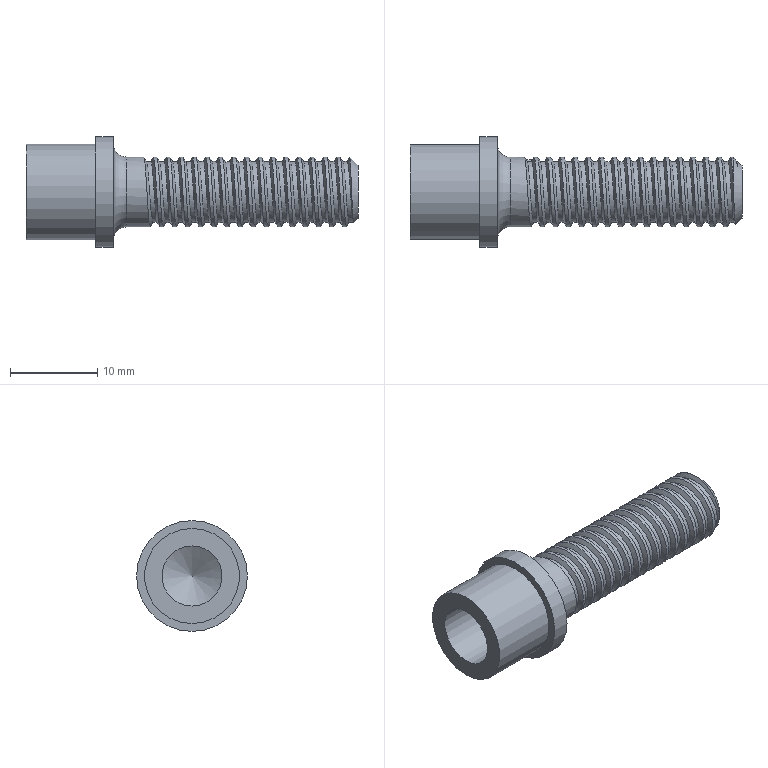Part | NX | features solid 2 | 1 solid | 30 faces | box 38.042 x 12.7 x 12.7 mm | volume 1971 mm3 | cylinder 20 | plane 5 | cone 2 | spline 2 | torus 1 | commonest cylinder face diameters 8.003 x16 6.9 x1 7 x1 10.9 x1 12.7 x1